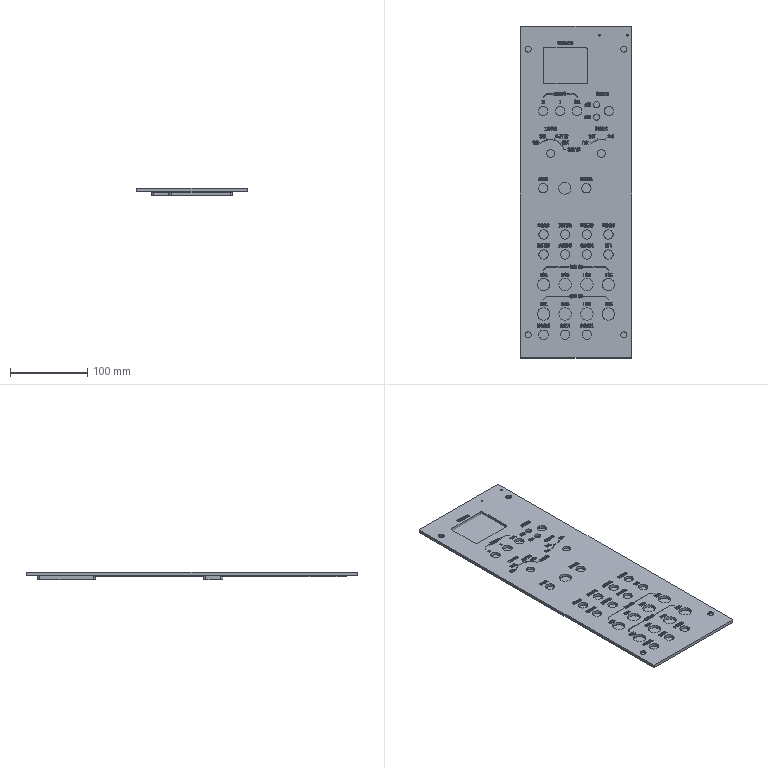NC program | Mastercam | posted with a generic post
Lines 8616 to 8664 of 54676:
(10 FEM |TOOL - 10|DIA. OFF. - 10|LEN. - 10|TOOL DIA. - 10.)
N7410 T10 M6
N7412 G0 G54 G90 X49. Y22. C0. B0. S7000 M3
N7414 G43 H10 Z50.
N7416 Z1.
N7418 G1 Z-5.95 F600.
N7420 Y21. F1000.
N7422 G3 X50. Y20. I1.
N7424 X63. Y33. J13.
N7426 X50. Y46. I-13.
N7428 X37. Y33. J-13.
N7430 X50. Y20. I13.
N7432 X51. Y21. J1.
N7434 G1 Y22.
N7436 G0 Z50.
N7438 X49. Y-44.
N7440 Z1.
N7442 G1 Z-5.95 F600.
N7444 Y-45. F1000.
N7446 G3 X50. Y-46. I1.
N7448 X63. Y-33. J13.
N7450 X50. Y-20. I-13.
N7452 X37. Y-33. J-13.
N7454 X50. Y-46. I13.
N7456 X51. Y-45. J1.
N7458 G1 Y-44.
N7460 G0 Z50.
N7462 X-215. Y79.5
N7464 Z1.
N7466 G1 Z-9.95 F600.
N7468 Y78.5 F1000.
N7470 G3 X-214. Y77.5 I1.
N7472 G1 X214.
N7474 G2 X220. Y71.5 J-6.
N7476 G1 Y-71.5
N7478 G2 X214. Y-77.5 I-6.
N7480 G1 X-214.
N7482 G2 X-220. Y-71.5 J6.
N7484 G1 Y71.5
N7486 G2 X-214. Y77.5 I6.
N7488 G3 X-213. Y78.5 J1.
N7490 G1 Y79.5
N7492 G0 Z50.
N7494 M5
N7496 G0 G28 G91 Z0.
N7498 G28
N7500 M01
N7502 G0 G17 G40 G80 G90 G94 G98
N7504 G0 G28 G91 Z0.